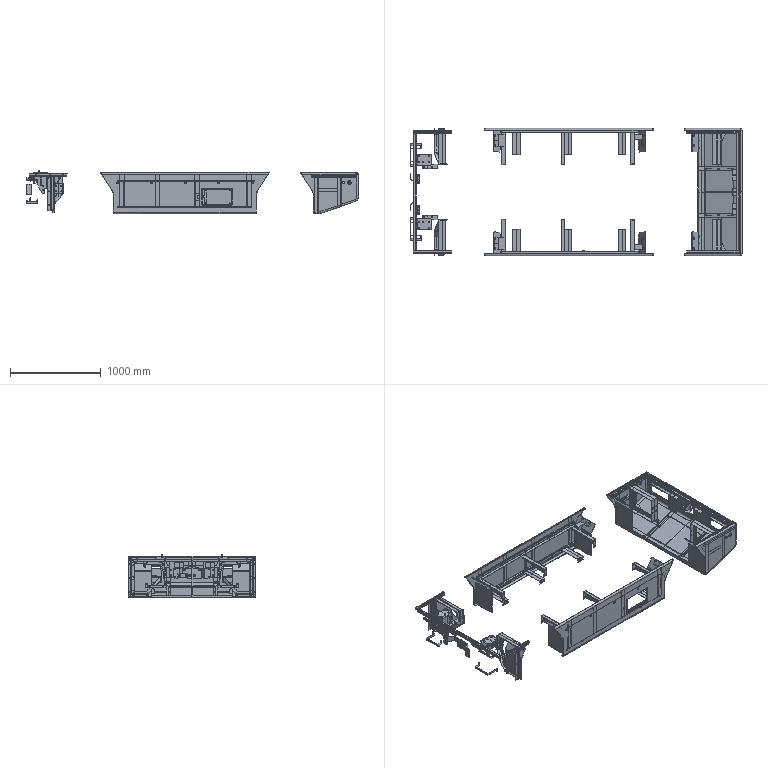Part | NX | features BREP 278 | 187 solids | 7068 faces | volume 31583893 mm3 | plane 3771 | cylinder 2099 | cone 704 | spline 408 | torus 84 | sphere 2 | commonest cylinder face diameters 8 x416 10 x254 13 x220 12 x190 11 x156 20 x130